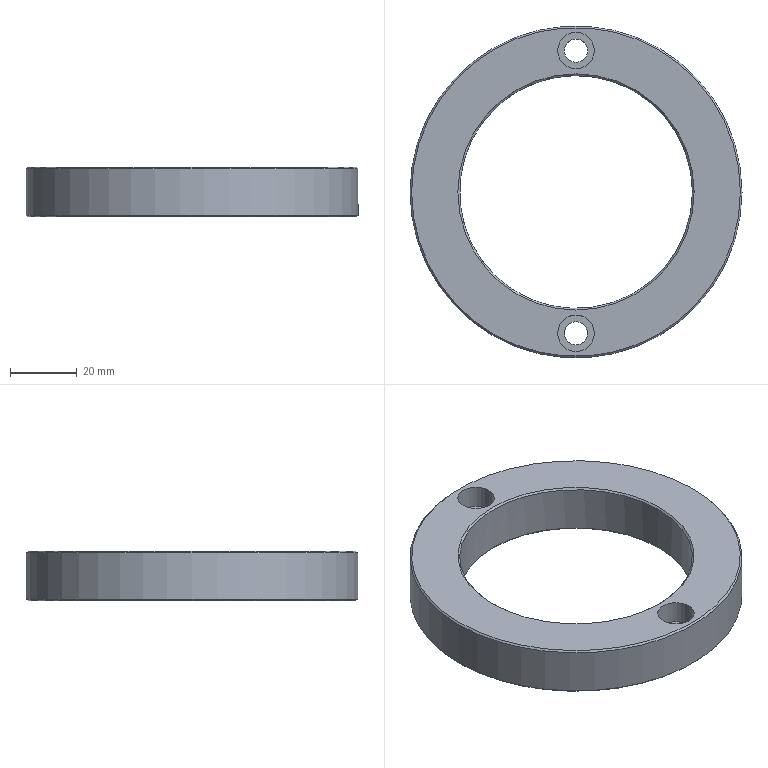Part | NX | features solid 2 | 1 solid | 14 faces | box 99.8 x 99.8 x 15 mm | volume 57533 mm3 | cylinder 6 | plane 4 | cone 4 | commonest cylinder face diameters 7 x2 11 x2 70 x1 99.8 x1
STEP:
#1=CARTESIAN_POINT('',(-3.5,42.5,170.5));
#2=VERTEX_POINT('',#1);
#3=CARTESIAN_POINT('',(0.,42.5,170.5));
#4=DIRECTION('',(0.,0.,1.));
#5=DIRECTION('',(-1.,0.,0.));
#6=AXIS2_PLACEMENT_3D('',#3,#4,#5);
#7=CIRCLE('',#6,3.5);
#8=EDGE_CURVE('',#2,#2,#7,.T.);
#9=ORIENTED_EDGE('',*,*,#8,.T.);
#10=EDGE_LOOP('',(#9));
#11=FACE_BOUND('',#10,.T.);
#12=CARTESIAN_POINT('',(-3.5,-42.5,170.5));
#13=VERTEX_POINT('',#12);
#14=CARTESIAN_POINT('',(0.,-42.5,170.5));
#15=DIRECTION('',(0.,0.,1.));
#16=DIRECTION('',(-1.,0.,0.));
#17=AXIS2_PLACEMENT_3D('',#14,#15,#16);
#18=CIRCLE('',#17,3.5);
#19=EDGE_CURVE('',#13,#13,#18,.T.);
#20=ORIENTED_EDGE('',*,*,#19,.T.);
#21=EDGE_LOOP('',(#20));
#22=FACE_BOUND('',#21,.T.);
#23=CARTESIAN_POINT('',(-35.5,0.,170.5));
#24=VERTEX_POINT('',#23);
#25=CARTESIAN_POINT('',(0.,0.,170.5));
#26=DIRECTION('',(0.,0.,-1.));
#27=DIRECTION('',(-1.,0.,0.));
#28=AXIS2_PLACEMENT_3D('',#25,#26,#27);
#29=CIRCLE('',#28,35.5);
#30=EDGE_CURVE('',#24,#24,#29,.F.);
#31=ORIENTED_EDGE('',*,*,#30,.T.);
#32=EDGE_LOOP('',(#31));
#33=FACE_BOUND('',#32,.T.);
#34=CARTESIAN_POINT('',(-49.4,0.,170.5));
#35=VERTEX_POINT('',#34);
#36=CARTESIAN_POINT('',(0.,0.,170.5));
#37=DIRECTION('',(0.,0.,-1.));
#38=DIRECTION('',(-1.,0.,0.));
#39=AXIS2_PLACEMENT_3D('',#36,#37,#38);
#40=CIRCLE('',#39,49.4);
#41=EDGE_CURVE('',#35,#35,#40,.T.);
#42=ORIENTED_EDGE('',*,*,#41,.T.);
#43=EDGE_LOOP('',(#42));
#44=FACE_BOUND('',#43,.T.);
#45=CARTESIAN_POINT('',(0.,0.,170.5));
#46=DIRECTION('',(0.,0.,-1.));
#47=DIRECTION('',(-1.,0.,0.));
#48=AXIS2_PLACEMENT_3D('',#45,#46,#47);
#49=PLANE('',#48);
#50=ADVANCED_FACE('',(#11,#22,#33,#44),#49,.T.);
#51=CARTESIAN_POINT('',(-5.5,42.5,185.5));
#52=VERTEX_POINT('',#51);
#53=CARTESIAN_POINT('',(0.,42.5,185.5));
#54=DIRECTION('',(0.,0.,-1.));
#55=DIRECTION('',(-1.,0.,0.));
#56=AXIS2_PLACEMENT_3D('',#53,#54,#55);
#57=CIRCLE('',#56,5.5);
#58=EDGE_CURVE('',#52,#52,#57,.T.);
#59=ORIENTED_EDGE('',*,*,#58,.T.);
#60=EDGE_LOOP('',(#59));
#61=FACE_BOUND('',#60,.T.);
#62=CARTESIAN_POINT('',(-5.5,-42.5,185.5));
#63=VERTEX_POINT('',#62);
#64=CARTESIAN_POINT('',(0.,-42.5,185.5));
#65=DIRECTION('',(0.,0.,-1.));
#66=DIRECTION('',(-1.,0.,0.));
#67=AXIS2_PLACEMENT_3D('',#64,#65,#66);
#68=CIRCLE('',#67,5.5);
#69=EDGE_CURVE('',#63,#63,#68,.T.);
#70=ORIENTED_EDGE('',*,*,#69,.T.);
#71=EDGE_LOOP('',(#70));
#72=FACE_BOUND('',#71,.T.);
#73=CARTESIAN_POINT('',(35.5,0.,185.5));
#74=VERTEX_POINT('',#73);
#75=CARTESIAN_POINT('',(0.,0.,185.5));
#76=DIRECTION('',(0.,0.,1.));
#77=DIRECTION('',(1.,0.,0.));
#78=AXIS2_PLACEMENT_3D('',#75,#76,#77);
#79=CIRCLE('',#78,35.5);
#80=EDGE_CURVE('',#74,#74,#79,.F.);
#81=ORIENTED_EDGE('',*,*,#80,.T.);
#82=EDGE_LOOP('',(#81));
#83=FACE_BOUND('',#82,.T.);
#84=CARTESIAN_POINT('',(49.4,0.,185.5));
#85=VERTEX_POINT('',#84);
#86=CARTESIAN_POINT('',(0.,0.,185.5));
#87=DIRECTION('',(0.,0.,1.));
#88=DIRECTION('',(1.,0.,0.));
#89=AXIS2_PLACEMENT_3D('',#86,#87,#88);
#90=CIRCLE('',#89,49.4);
#91=EDGE_CURVE('',#85,#85,#90,.T.);
#92=ORIENTED_EDGE('',*,*,#91,.T.);
#93=EDGE_LOOP('',(#92));
#94=FACE_BOUND('',#93,.T.);
#95=CARTESIAN_POINT('',(0.,0.,185.5));
#96=DIRECTION('',(0.,0.,1.));
#97=DIRECTION('',(1.,0.,0.));
#98=AXIS2_PLACEMENT_3D('',#95,#96,#97);
#99=PLANE('',#98);
#100=ADVANCED_FACE('',(#61,#72,#83,#94),#99,.T.);
#101=CARTESIAN_POINT('',(49.9,0.,185.));
#102=VERTEX_POINT('',#101);
#103=CARTESIAN_POINT('',(0.,0.,185.));
#104=DIRECTION('',(0.,0.,1.));
#105=DIRECTION('',(1.,0.,0.));
#106=AXIS2_PLACEMENT_3D('',#103,#104,#105);
#107=CIRCLE('',#106,49.9);
#108=EDGE_CURVE('',#102,#102,#107,.F.);
#109=ORIENTED_EDGE('',*,*,#108,.T.);
#110=EDGE_LOOP('',(#109));
#111=FACE_BOUND('',#110,.T.);
#112=CARTESIAN_POINT('',(-49.9,0.,171.));
#113=VERTEX_POINT('',#112);
#114=CARTESIAN_POINT('',(0.,0.,171.));
#115=DIRECTION('',(0.,0.,-1.));
#116=DIRECTION('',(-1.,0.,0.));
#117=AXIS2_PLACEMENT_3D('',#114,#115,#116);
#118=CIRCLE('',#117,49.9);
#119=EDGE_CURVE('',#113,#113,#118,.F.);
#120=ORIENTED_EDGE('',*,*,#119,.T.);
#121=EDGE_LOOP('',(#120));
#122=FACE_BOUND('',#121,.T.);
#123=CARTESIAN_POINT('',(0.,0.,185.5));
#124=DIRECTION('',(0.,0.,-1.));
#125=DIRECTION('',(1.,0.,0.));
#126=AXIS2_PLACEMENT_3D('',#123,#124,#125);
#127=CYLINDRICAL_SURFACE('',#126,49.9);
#128=ADVANCED_FACE('',(#111,#122),#127,.T.);
#129=ORIENTED_EDGE('',*,*,#91,.F.);
#130=EDGE_LOOP('',(#129));
#131=FACE_BOUND('',#130,.T.);
#132=ORIENTED_EDGE('',*,*,#108,.F.);
#133=EDGE_LOOP('',(#132));
#134=FACE_BOUND('',#133,.T.);
#135=CARTESIAN_POINT('',(0.,0.,185.));
#136=DIRECTION('',(0.,0.,-1.));
#137=DIRECTION('',(-1.,0.,0.));
#138=AXIS2_PLACEMENT_3D('',#135,#136,#137);
#139=CONICAL_SURFACE('',#138,49.9,0.7854);
#140=ADVANCED_FACE('',(#131,#134),#139,.T.);
#141=ORIENTED_EDGE('',*,*,#41,.F.);
#142=EDGE_LOOP('',(#141));
#143=FACE_BOUND('',#142,.T.);
#144=ORIENTED_EDGE('',*,*,#119,.F.);
#145=EDGE_LOOP('',(#144));
#146=FACE_BOUND('',#145,.T.);
#147=CARTESIAN_POINT('',(0.,0.,171.));
#148=DIRECTION('',(0.,0.,1.));
#149=DIRECTION('',(1.,0.,0.));
#150=AXIS2_PLACEMENT_3D('',#147,#148,#149);
#151=CONICAL_SURFACE('',#150,49.9,0.7854);
#152=ADVANCED_FACE('',(#143,#146),#151,.T.);
#153=CARTESIAN_POINT('',(35.,0.,185.));
#154=VERTEX_POINT('',#153);
#155=CARTESIAN_POINT('',(0.,0.,185.));
#156=DIRECTION('',(0.,0.,1.));
#157=DIRECTION('',(1.,0.,0.));
#158=AXIS2_PLACEMENT_3D('',#155,#156,#157);
#159=CIRCLE('',#158,35.);
#160=EDGE_CURVE('',#154,#154,#159,.T.);
#161=ORIENTED_EDGE('',*,*,#160,.T.);
#162=EDGE_LOOP('',(#161));
#163=FACE_BOUND('',#162,.T.);
#164=CARTESIAN_POINT('',(-35.,0.,171.));
#165=VERTEX_POINT('',#164);
#166=CARTESIAN_POINT('',(0.,0.,171.));
#167=DIRECTION('',(0.,0.,-1.));
#168=DIRECTION('',(-1.,0.,0.));
#169=AXIS2_PLACEMENT_3D('',#166,#167,#168);
#170=CIRCLE('',#169,35.);
#171=EDGE_CURVE('',#165,#165,#170,.T.);
#172=ORIENTED_EDGE('',*,*,#171,.T.);
#173=EDGE_LOOP('',(#172));
#174=FACE_BOUND('',#173,.T.);
#175=CARTESIAN_POINT('',(0.,0.,185.5));
#176=DIRECTION('',(0.,0.,-1.));
#177=DIRECTION('',(1.,0.,0.));
#178=AXIS2_PLACEMENT_3D('',#175,#176,#177);
#179=CYLINDRICAL_SURFACE('',#178,35.);
#180=ADVANCED_FACE('',(#163,#174),#179,.F.);
#181=ORIENTED_EDGE('',*,*,#160,.F.);
#182=EDGE_LOOP('',(#181));
#183=FACE_BOUND('',#182,.T.);
#184=ORIENTED_EDGE('',*,*,#80,.F.);
#185=EDGE_LOOP('',(#184));
#186=FACE_BOUND('',#185,.T.);
#187=CARTESIAN_POINT('',(0.,0.,185.5));
#188=DIRECTION('',(0.,0.,1.));
#189=DIRECTION('',(1.,0.,0.));
#190=AXIS2_PLACEMENT_3D('',#187,#188,#189);
#191=CONICAL_SURFACE('',#190,35.5,0.7854);
#192=ADVANCED_FACE('',(#183,#186),#191,.F.);
#193=ORIENTED_EDGE('',*,*,#171,.F.);
#194=EDGE_LOOP('',(#193));
#195=FACE_BOUND('',#194,.T.);
#196=ORIENTED_EDGE('',*,*,#30,.F.);
#197=EDGE_LOOP('',(#196));
#198=FACE_BOUND('',#197,.T.);
#199=CARTESIAN_POINT('',(0.,0.,170.5));
#200=DIRECTION('',(0.,0.,-1.));
#201=DIRECTION('',(-1.,0.,0.));
#202=AXIS2_PLACEMENT_3D('',#199,#200,#201);
#203=CONICAL_SURFACE('',#202,35.5,0.7854);
#204=ADVANCED_FACE('',(#195,#198),#203,.F.);
#205=CARTESIAN_POINT('',(-3.5,-42.5,178.5));
#206=VERTEX_POINT('',#205);
#207=CARTESIAN_POINT('',(0.,-42.5,178.5));
#208=DIRECTION('',(0.,0.,-1.));
#209=DIRECTION('',(-1.,0.,0.));
#210=AXIS2_PLACEMENT_3D('',#207,#208,#209);
#211=CIRCLE('',#210,3.5);
#212=EDGE_CURVE('',#206,#206,#211,.T.);
#213=ORIENTED_EDGE('',*,*,#212,.F.);
#214=EDGE_LOOP('',(#213));
#215=FACE_BOUND('',#214,.T.);
#216=ORIENTED_EDGE('',*,*,#19,.F.);
#217=EDGE_LOOP('',(#216));
#218=FACE_BOUND('',#217,.T.);
#219=CARTESIAN_POINT('',(0.,-42.5,170.5));
#220=DIRECTION('',(0.,0.,1.));
#221=DIRECTION('',(-1.,0.,0.));
#222=AXIS2_PLACEMENT_3D('',#219,#220,#221);
#223=CYLINDRICAL_SURFACE('',#222,3.5);
#224=ADVANCED_FACE('',(#215,#218),#223,.F.);
#225=ORIENTED_EDGE('',*,*,#212,.T.);
#226=EDGE_LOOP('',(#225));
#227=FACE_BOUND('',#226,.T.);
#228=CARTESIAN_POINT('',(-5.5,-42.5,178.5));
#229=VERTEX_POINT('',#228);
#230=CARTESIAN_POINT('',(0.,-42.5,178.5));
#231=DIRECTION('',(0.,0.,1.));
#232=DIRECTION('',(-1.,0.,0.));
#233=AXIS2_PLACEMENT_3D('',#230,#231,#232);
#234=CIRCLE('',#233,5.5);
#235=EDGE_CURVE('',#229,#229,#234,.F.);
#236=ORIENTED_EDGE('',*,*,#235,.F.);
#237=EDGE_LOOP('',(#236));
#238=FACE_BOUND('',#237,.T.);
#239=CARTESIAN_POINT('',(0.,-42.5,178.5));
#240=DIRECTION('',(0.,0.,-1.));
#241=DIRECTION('',(-1.,0.,0.));
#242=AXIS2_PLACEMENT_3D('',#239,#240,#241);
#243=PLANE('',#242);
#244=ADVANCED_FACE('',(#227,#238),#243,.F.);
#245=ORIENTED_EDGE('',*,*,#69,.F.);
#246=EDGE_LOOP('',(#245));
#247=FACE_BOUND('',#246,.T.);
#248=ORIENTED_EDGE('',*,*,#235,.T.);
#249=EDGE_LOOP('',(#248));
#250=FACE_BOUND('',#249,.T.);
#251=CARTESIAN_POINT('',(0.,-42.5,178.5));
#252=DIRECTION('',(0.,0.,1.));
#253=DIRECTION('',(-1.,0.,0.));
#254=AXIS2_PLACEMENT_3D('',#251,#252,#253);
#255=CYLINDRICAL_SURFACE('',#254,5.5);
#256=ADVANCED_FACE('',(#247,#250),#255,.F.);
#257=CARTESIAN_POINT('',(-3.5,42.5,178.5));
#258=VERTEX_POINT('',#257);
#259=CARTESIAN_POINT('',(0.,42.5,178.5));
#260=DIRECTION('',(0.,0.,-1.));
#261=DIRECTION('',(-1.,0.,0.));
#262=AXIS2_PLACEMENT_3D('',#259,#260,#261);
#263=CIRCLE('',#262,3.5);
#264=EDGE_CURVE('',#258,#258,#263,.T.);
#265=ORIENTED_EDGE('',*,*,#264,.F.);
#266=EDGE_LOOP('',(#265));
#267=FACE_BOUND('',#266,.T.);
#268=ORIENTED_EDGE('',*,*,#8,.F.);
#269=EDGE_LOOP('',(#268));
#270=FACE_BOUND('',#269,.T.);
#271=CARTESIAN_POINT('',(0.,42.5,170.5));
#272=DIRECTION('',(0.,0.,1.));
#273=DIRECTION('',(-1.,0.,0.));
#274=AXIS2_PLACEMENT_3D('',#271,#272,#273);
#275=CYLINDRICAL_SURFACE('',#274,3.5);
#276=ADVANCED_FACE('',(#267,#270),#275,.F.);
#277=ORIENTED_EDGE('',*,*,#264,.T.);
#278=EDGE_LOOP('',(#277));
#279=FACE_BOUND('',#278,.T.);
#280=CARTESIAN_POINT('',(-5.5,42.5,178.5));
#281=VERTEX_POINT('',#280);
#282=CARTESIAN_POINT('',(0.,42.5,178.5));
#283=DIRECTION('',(0.,0.,1.));
#284=DIRECTION('',(-1.,0.,0.));
#285=AXIS2_PLACEMENT_3D('',#282,#283,#284);
#286=CIRCLE('',#285,5.5);
#287=EDGE_CURVE('',#281,#281,#286,.F.);
#288=ORIENTED_EDGE('',*,*,#287,.F.);
#289=EDGE_LOOP('',(#288));
#290=FACE_BOUND('',#289,.T.);
#291=CARTESIAN_POINT('',(0.,42.5,178.5));
#292=DIRECTION('',(0.,0.,-1.));
#293=DIRECTION('',(-1.,0.,0.));
#294=AXIS2_PLACEMENT_3D('',#291,#292,#293);
#295=PLANE('',#294);
#296=ADVANCED_FACE('',(#279,#290),#295,.F.);
#297=ORIENTED_EDGE('',*,*,#58,.F.);
#298=EDGE_LOOP('',(#297));
#299=FACE_BOUND('',#298,.T.);
#300=ORIENTED_EDGE('',*,*,#287,.T.);
#301=EDGE_LOOP('',(#300));
#302=FACE_BOUND('',#301,.T.);
#303=CARTESIAN_POINT('',(0.,42.5,178.5));
#304=DIRECTION('',(0.,0.,1.));
#305=DIRECTION('',(-1.,0.,0.));
#306=AXIS2_PLACEMENT_3D('',#303,#304,#305);
#307=CYLINDRICAL_SURFACE('',#306,5.5);
#308=ADVANCED_FACE('',(#299,#302),#307,.F.);
#309=CLOSED_SHELL('',(#50,#100,#128,#140,#152,#180,#192,#204,#224,#244,#256,#276,#296,#308));
#310=MANIFOLD_SOLID_BREP('',#309);
#311=(LENGTH_UNIT()NAMED_UNIT(*)SI_UNIT(.MILLI.,.METRE.));
#312=UNCERTAINTY_MEASURE_WITH_UNIT(LENGTH_MEASURE(0.00001),#311,'','');
#313=(NAMED_UNIT(*)PLANE_ANGLE_UNIT()SI_UNIT($,.RADIAN.));
#314=(NAMED_UNIT(*)SI_UNIT($,.STERADIAN.)SOLID_ANGLE_UNIT());
#315=(GEOMETRIC_REPRESENTATION_CONTEXT(3)GLOBAL_UNCERTAINTY_ASSIGNED_CONTEXT((#312))GLOBAL_UNIT_ASSIGNED_CONTEXT((#311,#313,#314))REPRESENTATION_CONTEXT('',''));
#316=ADVANCED_BREP_SHAPE_REPRESENTATION('',(#310),#315);